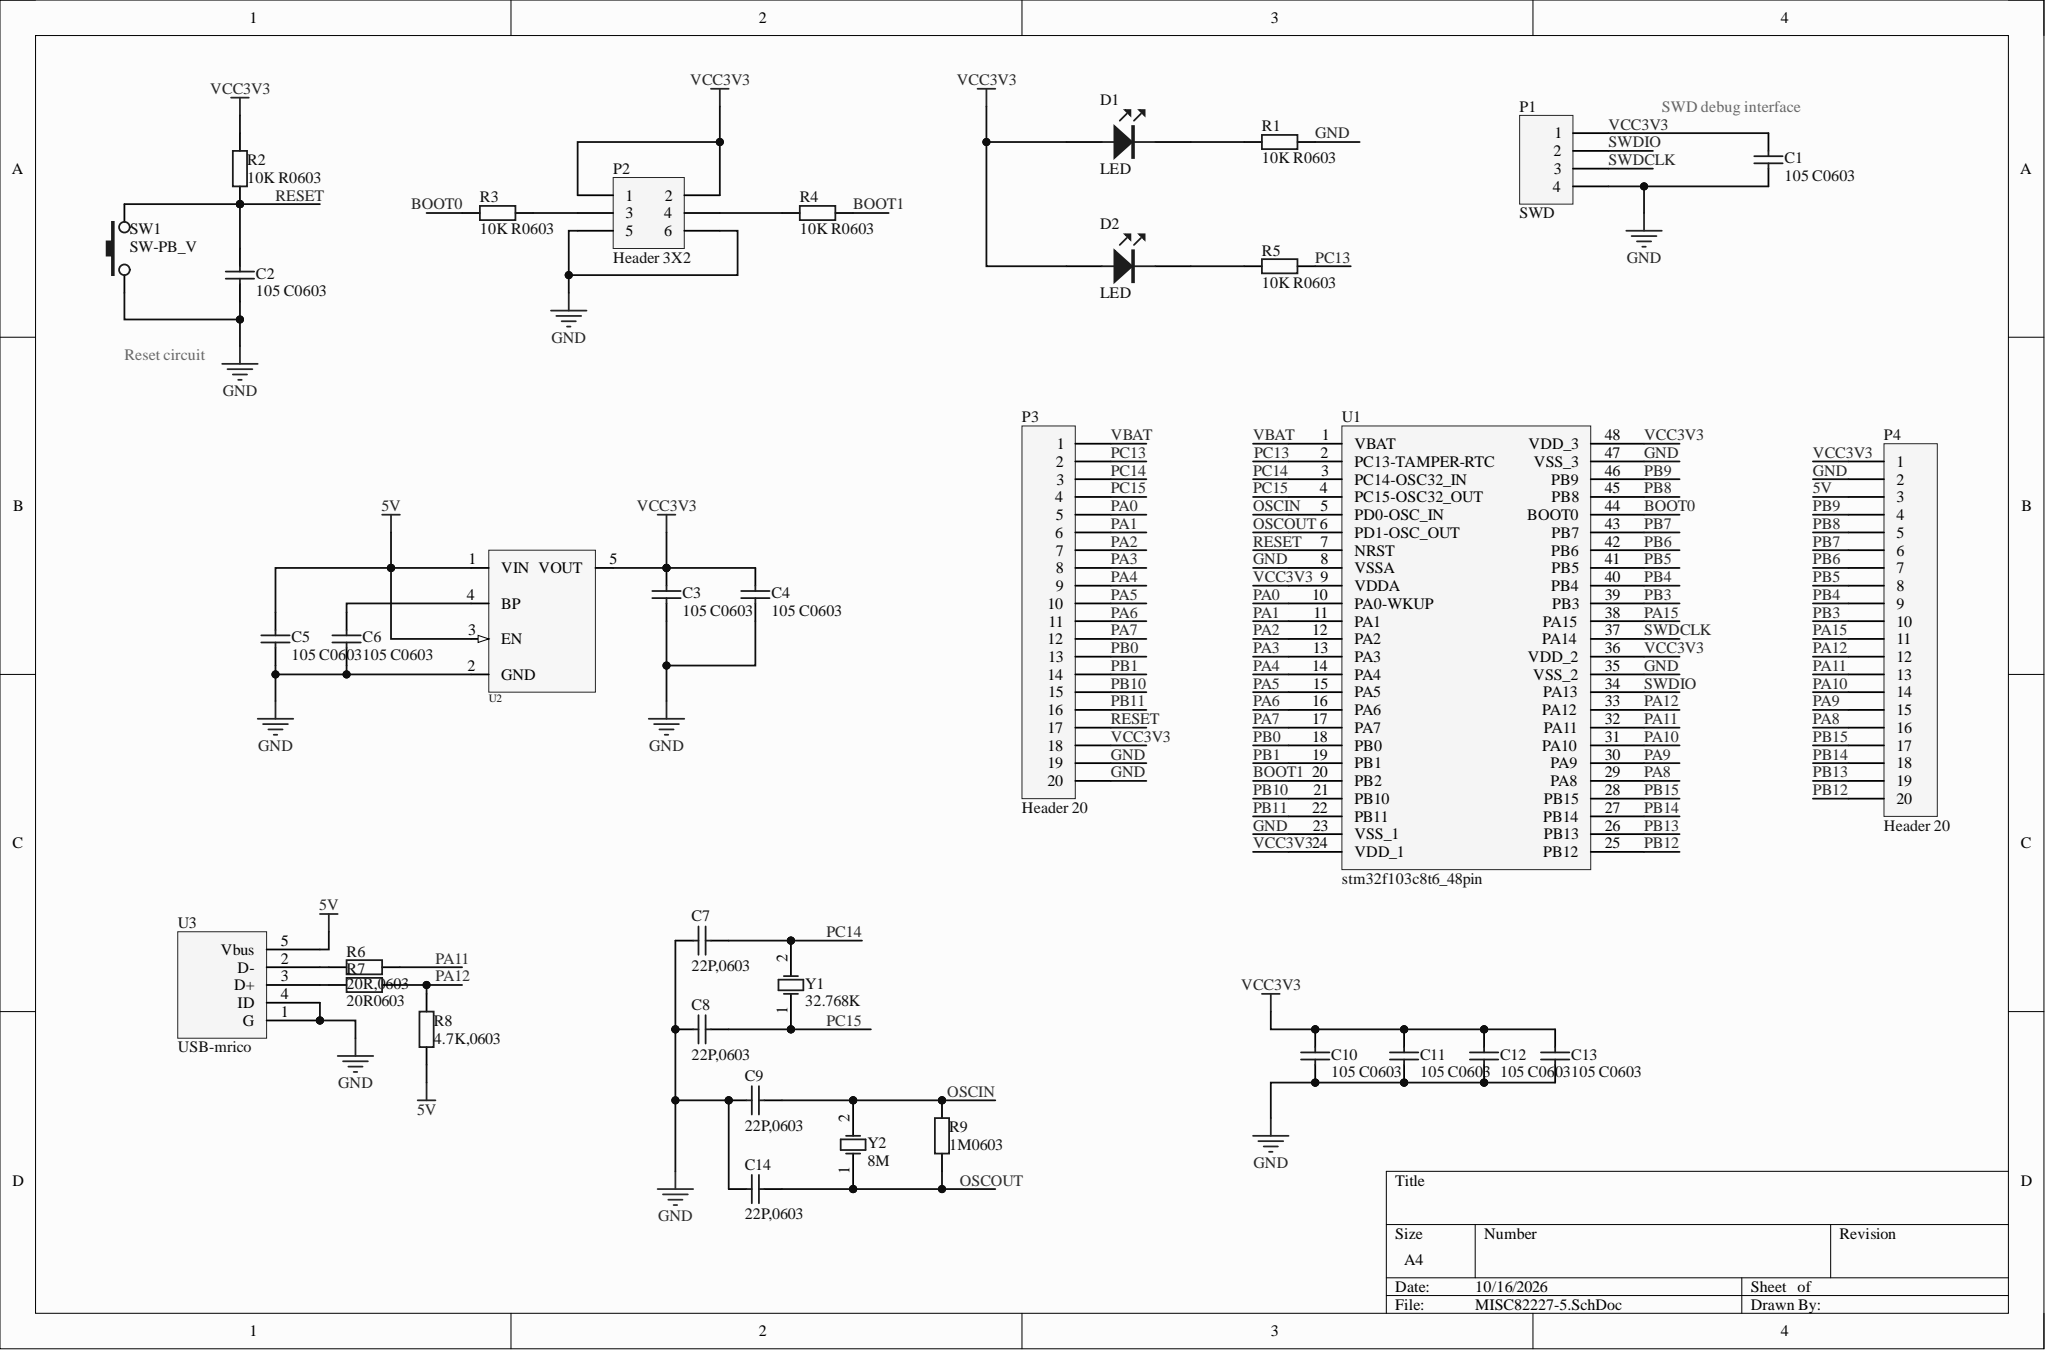Circuit board | Altium Designer | 35 parts | 50 nets
Bill of materials:
Comment,Description,Designator,Footprint,LibRef,Quantity
"105 C0603","","C1, C2, C3, C4, C5, C6, C10, C11, C12, C13","C 0603","Cap","10"
"22P,0603","Capacitor","C7, C8, C9, C14","C 0603","Cap","4"
"LED","","D1, D2","LED 0805G","LED","2"
"SWD","Header, 4-Pin","P1","HDR-1X4_H","Header 4","1"
"Header 3X2","Header, 3-Pin, Dual row","P2","HDR-3X2","Header 3X2","1"
"Header 20","Header, 20-Pin","P3, P4","HDR1X20","Header 20","2"
"10K R0603","","R1, R2, R3, R4, R5","R 0603","Res2","5"
"20R,0603","Resistor","R6","R 0603","Res2","1"
"20R0603","Resistor","R7","R 0603","Res2","1"
"4.7K,0603","Resistor","R8","R 0603","Res2","1"
"1M0603","Resistor","R9","R 0603","Res2","1"
"SW-PB_V","","SW1","TSW SMD-3*6*2.5","SW-PB_V","1"
"stm32f103c8t6_48pin","","U1","TQFP48 7x7_L","stm32f103c8t6_48pin","1"
"RT9193","","U2","SOT23-5L","RT9193X_5P","1"
"USB-mrico","","U3","USB-micro_B","usb-STM","1"
"32.768K","Crystal Oscillator","Y1","XTAL-49S DIP","XTAL","1"
"8M","Crystal Oscillator","Y2","XTAL-49S DIP","XTAL","1"
Netlist (Protel format):
[
C1
C 0603
105 C0603



]
[
C2
C 0603
105 C0603



]
[
C3
C 0603
105 C0603



]
[
C4
C 0603
105 C0603



]
[
C5
C 0603
105 C0603



]
[
C6
C 0603
105 C0603



]
[
C7
C 0603
22P,0603



]
[
C8
C 0603
22P,0603



]
[
C9
C 0603
22P,0603



]
[
C10
C 0603
105 C0603



]
[
C11
C 0603
105 C0603



]
[
C12
C 0603
105 C0603



]
[
C13
C 0603
105 C0603



]
[
C14
C 0603
22P,0603



]
[
D1
LED 0805G
LED



]
[
D2
LED 0805G
LED



]
[
P1
HDR-1X4_H
SWD



]
[
P2
HDR-3X2
Header 3X2



]
[
P3
HDR1X20
Header 20



]
[
P4
HDR1X20
Header 20



]
[
R1
R 0603
10K R0603



]
[
R2
R 0603
10K R0603



]
[
R3
R 0603
10K R0603



]
[
R4
R 0603
10K R0603



]
[
R5
R 0603
10K R0603



]
[
R6
R 0603
20R,0603



]
[
R7
R 0603
20R0603



]
[
R8
R 0603
4.7K,0603



]
[
R9
R 0603
1M0603



]
[
SW1
TSW SMD-3*6*2.5
SW-PB_V



]
[
U1
TQFP48 7x7_L
stm32f103c8t6_48pin



]
[
U2
SOT23-5L
RT9193



]
[
U3
USB-micro_B
USB-mrico



]
[
Y1
XTAL-49S DIP
32.768K



]
[
Y2
XTAL-49S DIP
8M



]
(
VCC3V3
C1-2
C3-2
C4-2
C10-2
C11-2
C12-2
C13-2
D1-1
D2-1
P1-1
P2-1
P2-2
P3-18
P4-1
R2-2
U1-9
U1-24
U1-36
U1-48
U2-5
)
(
VBAT
P3-1
U1-1
)
(
SWDIO
P1-2
U1-34
)
(
SWDCLK
P1-3
U1-37
)
(
RESET
C2-2
P3-17
R2-1
SW1-2
U1-7
)
(
PC15
C8-1
P3-4
U1-4
Y1-1
)
(
PC14
C7-1
P3-3
U1-3
Y1-2
)
(
PC13
P3-2
R5-2
U1-2
)
(
PB15
P4-17
U1-28
)
(
PB14
P4-18
U1-27
)
(
PB13
P4-19
U1-26
)
(
PB12
P4-20
U1-25
)
(
PB11
P3-16
U1-22
)
(
PB10
P3-15
U1-21
)
(
PB9
P4-4
U1-46
)
(
PB8
P4-5
U1-45
)
(
PB7
P4-6
U1-43
)
(
PB6
P4-7
U1-42
)
(
PB5
P4-8
U1-41
)
(
PB4
P4-9
U1-40
)
(
PB3
P4-10
U1-39
)
(
PB1
P3-14
U1-19
)
(
PB0
P3-13
U1-18
)
(
PA15
P4-11
U1-38
)
(
PA12
P4-12
R7-2
R8-2
U1-33
)
(
PA11
P4-13
R6-2
U1-32
)
(
PA10
P4-14
U1-31
)
(
PA9
P4-15
U1-30
)
(
PA8
P4-16
U1-29
)
(
PA7
P3-12
U1-17
)
(
PA6
P3-11
U1-16
)
(
PA5
P3-10
U1-15
)
(
PA4
P3-9
U1-14
)
(
PA3
P3-8
U1-13
)
(
PA2
P3-7
U1-12
)
(
PA1
P3-6
U1-11
)
(
PA0
P3-5
U1-10
)
(
OSCOUT
C14-1
R9-1
U1-6
Y2-1
)
(
OSCIN
C9-1
R9-2
U1-5
Y2-2
)
(
NetR7_1
R7-1
U3-3
)
(
NetR6_1
R6-1
U3-2
)
(
NetP2_4
P2-4
R4-1
)
(
NetP2_3
P2-3
R3-2
)
(
NetD2_2
D2-2
R5-1
)
(
NetD1_2
D1-2
R1-1
)
(
NetC6_2
C6-2
U2-4
)
(
GND
C1-1
C2-1
C3-1
C4-1
C5-1
C6-1
C7-2
C8-2
C9-2
C10-1
C11-1
C12-1
C13-1
C14-2
P1-4
P2-5
P2-6
P3-19
P3-20
P4-2
R1-2
SW1-1
U1-8
U1-23
U1-35
U1-47
U2-2
U3-1
U3-4
)
(
BOOT1
R4-2
U1-20
)
(
BOOT0
R3-1
U1-44
)
(
5V
C5-2
P4-3
R8-1
U2-1
U2-3
U3-5
)